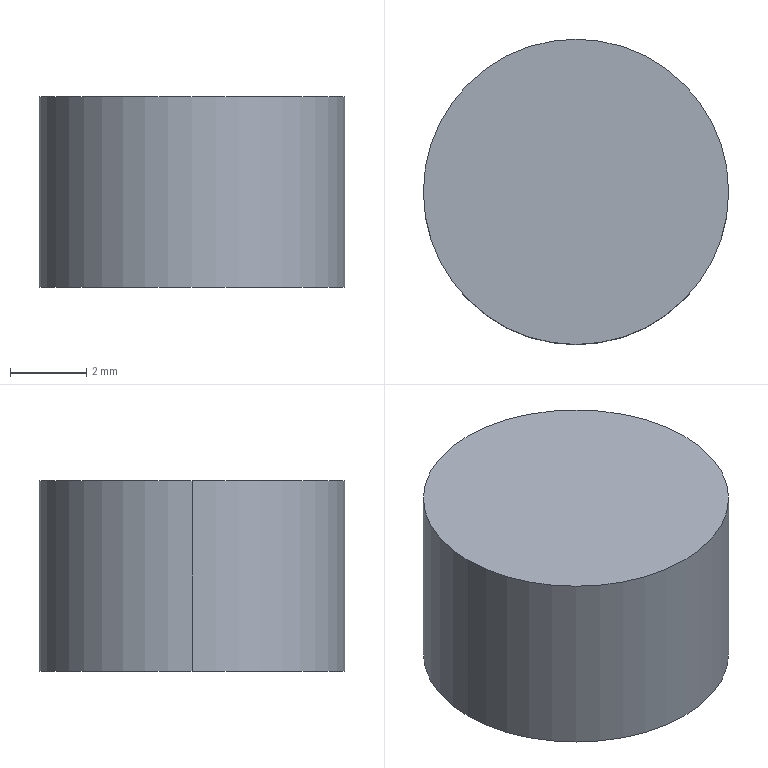Part | NX | features BREP 1 | 1 solid | 4 faces | box 8 x 8 x 5 mm | volume 251.327 mm3 | cylinder 2 | plane 2 | commonest cylinder face diameters 8 x2
STEP:
#1=CARTESIAN_POINT('',(200.354,29.098,-6.));
#2=VERTEX_POINT('',#1);
#3=CARTESIAN_POINT('',(208.354,29.098,-6.));
#4=VERTEX_POINT('',#3);
#5=CARTESIAN_POINT('',(204.354,29.098,-6.));
#6=DIRECTION('',(0.,0.,-1.));
#7=DIRECTION('',(1.,0.,0.));
#8=AXIS2_PLACEMENT_3D('',#5,#6,#7);
#9=CIRCLE('',#8,4.);
#10=EDGE_CURVE('',#2,#4,#9,.T.);
#11=ORIENTED_EDGE('',*,*,#10,.F.);
#12=CARTESIAN_POINT('',(200.354,29.098,-1.));
#13=VERTEX_POINT('',#12);
#14=CARTESIAN_POINT('',(200.354,29.098,-14.899));
#15=DIRECTION('',(0.,0.,1.));
#16=VECTOR('',#15,1000.);
#17=LINE('',#14,#16);
#18=EDGE_CURVE('',#2,#13,#17,.T.);
#19=ORIENTED_EDGE('',*,*,#18,.T.);
#20=CARTESIAN_POINT('',(208.354,29.098,-1.));
#21=VERTEX_POINT('',#20);
#22=CARTESIAN_POINT('',(204.354,29.098,-1.));
#23=DIRECTION('',(0.,0.,1.));
#24=DIRECTION('',(1.,0.,0.));
#25=AXIS2_PLACEMENT_3D('',#22,#23,#24);
#26=CIRCLE('',#25,4.);
#27=EDGE_CURVE('',#21,#13,#26,.T.);
#28=ORIENTED_EDGE('',*,*,#27,.F.);
#29=CARTESIAN_POINT('',(208.354,29.098,-14.899));
#30=DIRECTION('',(0.,0.,1.));
#31=VECTOR('',#30,1000.);
#32=LINE('',#29,#31);
#33=EDGE_CURVE('',#4,#21,#32,.T.);
#34=ORIENTED_EDGE('',*,*,#33,.F.);
#35=EDGE_LOOP('',(#11,#19,#28,#34));
#36=FACE_BOUND('',#35,.T.);
#37=CARTESIAN_POINT('',(204.354,29.098,-14.899));
#38=DIRECTION('',(0.,0.,1.));
#39=DIRECTION('',(-1.,0.,0.));
#40=AXIS2_PLACEMENT_3D('',#37,#38,#39);
#41=CYLINDRICAL_SURFACE('',#40,4.);
#42=ADVANCED_FACE('',(#36),#41,.T.);
#43=ORIENTED_EDGE('',*,*,#18,.F.);
#44=CARTESIAN_POINT('',(204.354,29.098,-6.));
#45=DIRECTION('',(0.,0.,-1.));
#46=DIRECTION('',(1.,0.,0.));
#47=AXIS2_PLACEMENT_3D('',#44,#45,#46);
#48=CIRCLE('',#47,4.);
#49=EDGE_CURVE('',#4,#2,#48,.T.);
#50=ORIENTED_EDGE('',*,*,#49,.F.);
#51=ORIENTED_EDGE('',*,*,#33,.T.);
#52=CARTESIAN_POINT('',(204.354,29.098,-1.));
#53=DIRECTION('',(0.,0.,1.));
#54=DIRECTION('',(1.,0.,0.));
#55=AXIS2_PLACEMENT_3D('',#52,#53,#54);
#56=CIRCLE('',#55,4.);
#57=EDGE_CURVE('',#13,#21,#56,.T.);
#58=ORIENTED_EDGE('',*,*,#57,.F.);
#59=EDGE_LOOP('',(#43,#50,#51,#58));
#60=FACE_BOUND('',#59,.T.);
#61=CARTESIAN_POINT('',(204.354,29.098,-14.899));
#62=DIRECTION('',(0.,0.,1.));
#63=DIRECTION('',(-1.,0.,0.));
#64=AXIS2_PLACEMENT_3D('',#61,#62,#63);
#65=CYLINDRICAL_SURFACE('',#64,4.);
#66=ADVANCED_FACE('',(#60),#65,.T.);
#67=ORIENTED_EDGE('',*,*,#27,.T.);
#68=ORIENTED_EDGE('',*,*,#57,.T.);
#69=EDGE_LOOP('',(#67,#68));
#70=FACE_BOUND('',#69,.T.);
#71=CARTESIAN_POINT('',(204.354,29.098,-1.));
#72=DIRECTION('',(0.,0.,1.));
#73=DIRECTION('',(-1.,0.,0.));
#74=AXIS2_PLACEMENT_3D('',#71,#72,#73);
#75=PLANE('',#74);
#76=ADVANCED_FACE('',(#70),#75,.T.);
#77=ORIENTED_EDGE('',*,*,#49,.T.);
#78=ORIENTED_EDGE('',*,*,#10,.T.);
#79=EDGE_LOOP('',(#77,#78));
#80=FACE_BOUND('',#79,.T.);
#81=CARTESIAN_POINT('',(204.354,29.098,-6.));
#82=DIRECTION('',(0.,0.,1.));
#83=DIRECTION('',(-1.,0.,0.));
#84=AXIS2_PLACEMENT_3D('',#81,#82,#83);
#85=PLANE('',#84);
#86=ADVANCED_FACE('',(#80),#85,.F.);
#87=CLOSED_SHELL('',(#42,#66,#76,#86));
#88=MANIFOLD_SOLID_BREP('',#87);
#89=(LENGTH_UNIT()NAMED_UNIT(*)SI_UNIT(.MILLI.,.METRE.));
#90=UNCERTAINTY_MEASURE_WITH_UNIT(LENGTH_MEASURE(0.00001),#89,'','');
#91=(NAMED_UNIT(*)PLANE_ANGLE_UNIT()SI_UNIT($,.RADIAN.));
#92=(NAMED_UNIT(*)SI_UNIT($,.STERADIAN.)SOLID_ANGLE_UNIT());
#93=(GEOMETRIC_REPRESENTATION_CONTEXT(3)GLOBAL_UNCERTAINTY_ASSIGNED_CONTEXT((#90))GLOBAL_UNIT_ASSIGNED_CONTEXT((#89,#91,#92))REPRESENTATION_CONTEXT('',''));
#94=ADVANCED_BREP_SHAPE_REPRESENTATION('',(#88),#93);